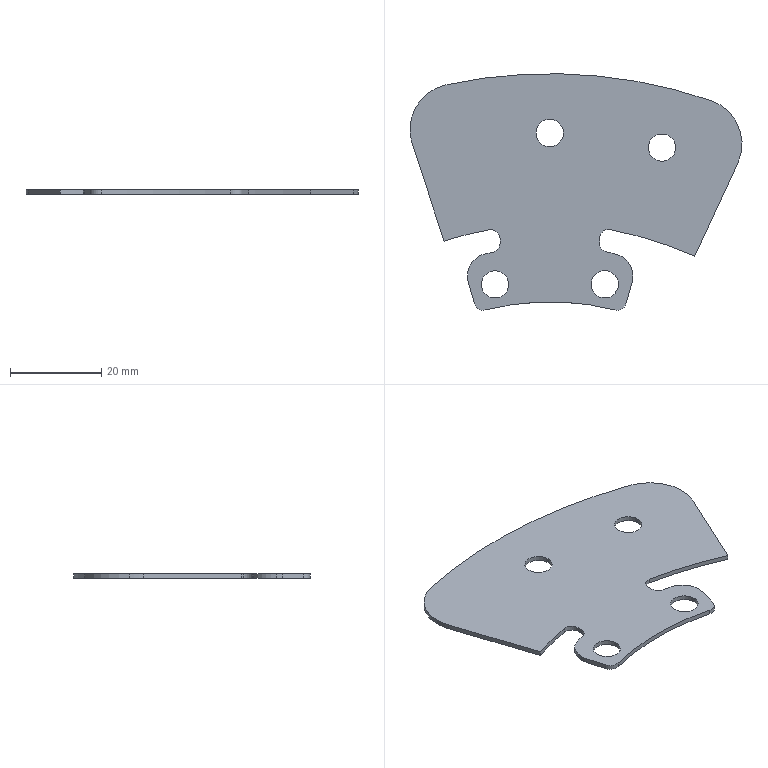Part | SolidWorks | features Extrusion 1 | 1 solid | 35 faces | box 72.756 x 51.823 x 1 mm | volume 2634 mm3 | cylinder 27 | plane 8 | commonest cylinder face diameters 6 x8 4 x7 10 x3 20 x3 140 x2 116 x1
STEP:
#1=CARTESIAN_POINT('',(21.592,11.76,1.));
#2=VERTEX_POINT('',#1);
#3=CARTESIAN_POINT('',(27.592,11.76,1.));
#4=VERTEX_POINT('',#3);
#5=CARTESIAN_POINT('',(24.592,11.76,1.));
#6=DIRECTION('',(0.,0.,1.));
#7=DIRECTION('',(1.,0.,0.));
#8=AXIS2_PLACEMENT_3D('',#5,#6,#7);
#9=CIRCLE('',#8,3.);
#10=EDGE_CURVE('',#2,#4,#9,.T.);
#11=ORIENTED_EDGE('',*,*,#10,.T.);
#12=CARTESIAN_POINT('',(27.592,11.76,0.));
#13=VERTEX_POINT('',#12);
#14=CARTESIAN_POINT('',(27.592,11.76,1.));
#15=DIRECTION('',(0.,0.,-1.));
#16=VECTOR('',#15,1000.);
#17=LINE('',#14,#16);
#18=EDGE_CURVE('',#4,#13,#17,.T.);
#19=ORIENTED_EDGE('',*,*,#18,.T.);
#20=CARTESIAN_POINT('',(21.592,11.76,0.));
#21=VERTEX_POINT('',#20);
#22=CARTESIAN_POINT('',(24.592,11.76,0.));
#23=DIRECTION('',(0.,0.,1.));
#24=DIRECTION('',(1.,0.,0.));
#25=AXIS2_PLACEMENT_3D('',#22,#23,#24);
#26=CIRCLE('',#25,3.);
#27=EDGE_CURVE('',#21,#13,#26,.T.);
#28=ORIENTED_EDGE('',*,*,#27,.F.);
#29=CARTESIAN_POINT('',(21.592,11.76,1.));
#30=DIRECTION('',(0.,0.,-1.));
#31=VECTOR('',#30,1000.);
#32=LINE('',#29,#31);
#33=EDGE_CURVE('',#2,#21,#32,.T.);
#34=ORIENTED_EDGE('',*,*,#33,.F.);
#35=EDGE_LOOP('',(#11,#19,#28,#34));
#36=FACE_OUTER_BOUND('',#35,.T.);
#37=CARTESIAN_POINT('',(24.592,11.76,1.));
#38=DIRECTION('',(0.,0.,-1.));
#39=DIRECTION('',(-1.,0.,0.));
#40=AXIS2_PLACEMENT_3D('',#37,#38,#39);
#41=CYLINDRICAL_SURFACE('',#40,3.);
#42=ADVANCED_FACE('',(#36),#41,.F.);
#43=CARTESIAN_POINT('',(-3.,14.968,1.));
#44=VERTEX_POINT('',#43);
#45=CARTESIAN_POINT('',(3.,14.968,1.));
#46=VERTEX_POINT('',#45);
#47=CARTESIAN_POINT('',(0.,14.968,1.));
#48=DIRECTION('',(0.,0.,1.));
#49=DIRECTION('',(1.,0.,0.));
#50=AXIS2_PLACEMENT_3D('',#47,#48,#49);
#51=CIRCLE('',#50,3.);
#52=EDGE_CURVE('',#44,#46,#51,.T.);
#53=ORIENTED_EDGE('',*,*,#52,.T.);
#54=CARTESIAN_POINT('',(3.,14.968,0.));
#55=VERTEX_POINT('',#54);
#56=CARTESIAN_POINT('',(3.,14.968,1.));
#57=DIRECTION('',(0.,0.,-1.));
#58=VECTOR('',#57,1000.);
#59=LINE('',#56,#58);
#60=EDGE_CURVE('',#46,#55,#59,.T.);
#61=ORIENTED_EDGE('',*,*,#60,.T.);
#62=CARTESIAN_POINT('',(-3.,14.968,0.));
#63=VERTEX_POINT('',#62);
#64=CARTESIAN_POINT('',(0.,14.968,0.));
#65=DIRECTION('',(0.,0.,1.));
#66=DIRECTION('',(1.,0.,0.));
#67=AXIS2_PLACEMENT_3D('',#64,#65,#66);
#68=CIRCLE('',#67,3.);
#69=EDGE_CURVE('',#63,#55,#68,.T.);
#70=ORIENTED_EDGE('',*,*,#69,.F.);
#71=CARTESIAN_POINT('',(-3.,14.968,1.));
#72=DIRECTION('',(0.,0.,-1.));
#73=VECTOR('',#72,1000.);
#74=LINE('',#71,#73);
#75=EDGE_CURVE('',#44,#63,#74,.T.);
#76=ORIENTED_EDGE('',*,*,#75,.F.);
#77=EDGE_LOOP('',(#53,#61,#70,#76));
#78=FACE_OUTER_BOUND('',#77,.T.);
#79=CARTESIAN_POINT('',(0.,14.968,1.));
#80=DIRECTION('',(0.,0.,-1.));
#81=DIRECTION('',(-1.,0.,0.));
#82=AXIS2_PLACEMENT_3D('',#79,#80,#81);
#83=CYLINDRICAL_SURFACE('',#82,3.);
#84=ADVANCED_FACE('',(#78),#83,.F.);
#85=CARTESIAN_POINT('',(-14.981,-18.204,1.));
#86=VERTEX_POINT('',#85);
#87=CARTESIAN_POINT('',(-8.981,-18.204,1.));
#88=VERTEX_POINT('',#87);
#89=CARTESIAN_POINT('',(-11.981,-18.204,1.));
#90=DIRECTION('',(0.,0.,1.));
#91=DIRECTION('',(1.,0.,0.));
#92=AXIS2_PLACEMENT_3D('',#89,#90,#91);
#93=CIRCLE('',#92,3.);
#94=EDGE_CURVE('',#86,#88,#93,.T.);
#95=ORIENTED_EDGE('',*,*,#94,.T.);
#96=CARTESIAN_POINT('',(-8.981,-18.204,0.));
#97=VERTEX_POINT('',#96);
#98=CARTESIAN_POINT('',(-8.981,-18.204,1.));
#99=DIRECTION('',(0.,0.,-1.));
#100=VECTOR('',#99,1000.);
#101=LINE('',#98,#100);
#102=EDGE_CURVE('',#88,#97,#101,.T.);
#103=ORIENTED_EDGE('',*,*,#102,.T.);
#104=CARTESIAN_POINT('',(-14.981,-18.204,0.));
#105=VERTEX_POINT('',#104);
#106=CARTESIAN_POINT('',(-11.981,-18.204,0.));
#107=DIRECTION('',(0.,0.,1.));
#108=DIRECTION('',(1.,0.,0.));
#109=AXIS2_PLACEMENT_3D('',#106,#107,#108);
#110=CIRCLE('',#109,3.);
#111=EDGE_CURVE('',#105,#97,#110,.T.);
#112=ORIENTED_EDGE('',*,*,#111,.F.);
#113=CARTESIAN_POINT('',(-14.981,-18.204,1.));
#114=DIRECTION('',(0.,0.,-1.));
#115=VECTOR('',#114,1000.);
#116=LINE('',#113,#115);
#117=EDGE_CURVE('',#86,#105,#116,.T.);
#118=ORIENTED_EDGE('',*,*,#117,.F.);
#119=EDGE_LOOP('',(#95,#103,#112,#118));
#120=FACE_OUTER_BOUND('',#119,.T.);
#121=CARTESIAN_POINT('',(-11.981,-18.204,1.));
#122=DIRECTION('',(0.,0.,-1.));
#123=DIRECTION('',(-1.,0.,0.));
#124=AXIS2_PLACEMENT_3D('',#121,#122,#123);
#125=CYLINDRICAL_SURFACE('',#124,3.);
#126=ADVANCED_FACE('',(#120),#125,.F.);
#127=CARTESIAN_POINT('',(9.061,-18.175,1.));
#128=VERTEX_POINT('',#127);
#129=CARTESIAN_POINT('',(15.061,-18.175,1.));
#130=VERTEX_POINT('',#129);
#131=CARTESIAN_POINT('',(12.061,-18.175,1.));
#132=DIRECTION('',(0.,0.,1.));
#133=DIRECTION('',(1.,0.,0.));
#134=AXIS2_PLACEMENT_3D('',#131,#132,#133);
#135=CIRCLE('',#134,3.);
#136=EDGE_CURVE('',#128,#130,#135,.T.);
#137=ORIENTED_EDGE('',*,*,#136,.T.);
#138=CARTESIAN_POINT('',(15.061,-18.175,0.));
#139=VERTEX_POINT('',#138);
#140=CARTESIAN_POINT('',(15.061,-18.175,1.));
#141=DIRECTION('',(0.,0.,-1.));
#142=VECTOR('',#141,1000.);
#143=LINE('',#140,#142);
#144=EDGE_CURVE('',#130,#139,#143,.T.);
#145=ORIENTED_EDGE('',*,*,#144,.T.);
#146=CARTESIAN_POINT('',(9.061,-18.175,0.));
#147=VERTEX_POINT('',#146);
#148=CARTESIAN_POINT('',(12.061,-18.175,0.));
#149=DIRECTION('',(0.,0.,1.));
#150=DIRECTION('',(1.,0.,0.));
#151=AXIS2_PLACEMENT_3D('',#148,#149,#150);
#152=CIRCLE('',#151,3.);
#153=EDGE_CURVE('',#147,#139,#152,.T.);
#154=ORIENTED_EDGE('',*,*,#153,.F.);
#155=CARTESIAN_POINT('',(9.061,-18.175,1.));
#156=DIRECTION('',(0.,0.,-1.));
#157=VECTOR('',#156,1000.);
#158=LINE('',#155,#157);
#159=EDGE_CURVE('',#128,#147,#158,.T.);
#160=ORIENTED_EDGE('',*,*,#159,.F.);
#161=EDGE_LOOP('',(#137,#145,#154,#160));
#162=FACE_OUTER_BOUND('',#161,.T.);
#163=CARTESIAN_POINT('',(12.061,-18.175,1.));
#164=DIRECTION('',(0.,0.,-1.));
#165=DIRECTION('',(-1.,0.,0.));
#166=AXIS2_PLACEMENT_3D('',#163,#164,#165);
#167=CYLINDRICAL_SURFACE('',#166,3.);
#168=ADVANCED_FACE('',(#162),#167,.F.);
#169=CARTESIAN_POINT('',(10.942,-8.168,1.));
#170=VERTEX_POINT('',#169);
#171=CARTESIAN_POINT('',(13.293,-6.199,1.));
#172=VERTEX_POINT('',#171);
#173=CARTESIAN_POINT('',(12.942,-8.168,1.));
#174=DIRECTION('',(0.,0.,-1.));
#175=DIRECTION('',(1.,0.,0.));
#176=AXIS2_PLACEMENT_3D('',#173,#174,#175);
#177=CIRCLE('',#176,2.);
#178=EDGE_CURVE('',#170,#172,#177,.T.);
#179=ORIENTED_EDGE('',*,*,#178,.F.);
#180=CARTESIAN_POINT('',(10.942,-8.168,0.));
#181=VERTEX_POINT('',#180);
#182=CARTESIAN_POINT('',(10.942,-8.168,1.));
#183=DIRECTION('',(0.,0.,-1.));
#184=VECTOR('',#183,1000.);
#185=LINE('',#182,#184);
#186=EDGE_CURVE('',#170,#181,#185,.T.);
#187=ORIENTED_EDGE('',*,*,#186,.T.);
#188=CARTESIAN_POINT('',(13.293,-6.199,0.));
#189=VERTEX_POINT('',#188);
#190=CARTESIAN_POINT('',(12.942,-8.168,0.));
#191=DIRECTION('',(0.,0.,-1.));
#192=DIRECTION('',(1.,0.,0.));
#193=AXIS2_PLACEMENT_3D('',#190,#191,#192);
#194=CIRCLE('',#193,2.);
#195=EDGE_CURVE('',#181,#189,#194,.T.);
#196=ORIENTED_EDGE('',*,*,#195,.T.);
#197=CARTESIAN_POINT('',(13.293,-6.199,1.));
#198=DIRECTION('',(0.,0.,-1.));
#199=VECTOR('',#198,1000.);
#200=LINE('',#197,#199);
#201=EDGE_CURVE('',#172,#189,#200,.T.);
#202=ORIENTED_EDGE('',*,*,#201,.F.);
#203=EDGE_LOOP('',(#179,#187,#196,#202));
#204=FACE_OUTER_BOUND('',#203,.T.);
#205=CARTESIAN_POINT('',(12.942,-8.168,1.));
#206=DIRECTION('',(0.,0.,-1.));
#207=DIRECTION('',(-1.,0.,0.));
#208=AXIS2_PLACEMENT_3D('',#205,#206,#207);
#209=CYLINDRICAL_SURFACE('',#208,2.);
#210=ADVANCED_FACE('',(#204),#209,.F.);
#211=CARTESIAN_POINT('',(-18.02,-16.372,1.));
#212=VERTEX_POINT('',#211);
#213=CARTESIAN_POINT('',(-17.824,-17.756,1.));
#214=VERTEX_POINT('',#213);
#215=CARTESIAN_POINT('',(-13.02,-16.372,1.));
#216=DIRECTION('',(0.,0.,1.));
#217=DIRECTION('',(1.,0.,0.));
#218=AXIS2_PLACEMENT_3D('',#215,#216,#217);
#219=CIRCLE('',#218,5.);
#220=EDGE_CURVE('',#212,#214,#219,.T.);
#221=ORIENTED_EDGE('',*,*,#220,.F.);
#222=CARTESIAN_POINT('',(-18.02,-16.372,0.));
#223=VERTEX_POINT('',#222);
#224=CARTESIAN_POINT('',(-18.02,-16.372,1.));
#225=DIRECTION('',(0.,0.,-1.));
#226=VECTOR('',#225,1000.);
#227=LINE('',#224,#226);
#228=EDGE_CURVE('',#212,#223,#227,.T.);
#229=ORIENTED_EDGE('',*,*,#228,.T.);
#230=CARTESIAN_POINT('',(-17.824,-17.756,0.));
#231=VERTEX_POINT('',#230);
#232=CARTESIAN_POINT('',(-13.02,-16.372,0.));
#233=DIRECTION('',(0.,0.,1.));
#234=DIRECTION('',(1.,0.,0.));
#235=AXIS2_PLACEMENT_3D('',#232,#233,#234);
#236=CIRCLE('',#235,5.);
#237=EDGE_CURVE('',#223,#231,#236,.T.);
#238=ORIENTED_EDGE('',*,*,#237,.T.);
#239=CARTESIAN_POINT('',(-17.824,-17.756,1.));
#240=DIRECTION('',(0.,0.,-1.));
#241=VECTOR('',#240,1000.);
#242=LINE('',#239,#241);
#243=EDGE_CURVE('',#214,#231,#242,.T.);
#244=ORIENTED_EDGE('',*,*,#243,.F.);
#245=EDGE_LOOP('',(#221,#229,#238,#244));
#246=FACE_OUTER_BOUND('',#245,.T.);
#247=CARTESIAN_POINT('',(-13.02,-16.372,1.));
#248=DIRECTION('',(0.,0.,-1.));
#249=DIRECTION('',(-1.,0.,0.));
#250=AXIS2_PLACEMENT_3D('',#247,#248,#249);
#251=CYLINDRICAL_SURFACE('',#250,5.);
#252=ADVANCED_FACE('',(#246),#251,.T.);
#253=CARTESIAN_POINT('',(-30.616,15.751,1.));
#254=VERTEX_POINT('',#253);
#255=CARTESIAN_POINT('',(-30.123,12.649,1.));
#256=VERTEX_POINT('',#255);
#257=CARTESIAN_POINT('',(-20.616,15.751,1.));
#258=DIRECTION('',(0.,0.,1.));
#259=DIRECTION('',(1.,0.,0.));
#260=AXIS2_PLACEMENT_3D('',#257,#258,#259);
#261=CIRCLE('',#260,10.);
#262=EDGE_CURVE('',#254,#256,#261,.T.);
#263=ORIENTED_EDGE('',*,*,#262,.F.);
#264=CARTESIAN_POINT('',(-30.616,15.751,0.));
#265=VERTEX_POINT('',#264);
#266=CARTESIAN_POINT('',(-30.616,15.751,1.));
#267=DIRECTION('',(0.,0.,-1.));
#268=VECTOR('',#267,1000.);
#269=LINE('',#266,#268);
#270=EDGE_CURVE('',#254,#265,#269,.T.);
#271=ORIENTED_EDGE('',*,*,#270,.T.);
#272=CARTESIAN_POINT('',(-30.123,12.649,0.));
#273=VERTEX_POINT('',#272);
#274=CARTESIAN_POINT('',(-20.616,15.751,0.));
#275=DIRECTION('',(0.,0.,1.));
#276=DIRECTION('',(1.,0.,0.));
#277=AXIS2_PLACEMENT_3D('',#274,#275,#276);
#278=CIRCLE('',#277,10.);
#279=EDGE_CURVE('',#265,#273,#278,.T.);
#280=ORIENTED_EDGE('',*,*,#279,.T.);
#281=CARTESIAN_POINT('',(-30.123,12.649,1.));
#282=DIRECTION('',(0.,0.,-1.));
#283=VECTOR('',#282,1000.);
#284=LINE('',#281,#283);
#285=EDGE_CURVE('',#256,#273,#284,.T.);
#286=ORIENTED_EDGE('',*,*,#285,.F.);
#287=EDGE_LOOP('',(#263,#271,#280,#286));
#288=FACE_OUTER_BOUND('',#287,.T.);
#289=CARTESIAN_POINT('',(-20.616,15.751,1.));
#290=DIRECTION('',(0.,0.,-1.));
#291=DIRECTION('',(-1.,0.,0.));
#292=AXIS2_PLACEMENT_3D('',#289,#290,#291);
#293=CYLINDRICAL_SURFACE('',#292,10.);
#294=ADVANCED_FACE('',(#288),#293,.T.);
#295=ORIENTED_EDGE('',*,*,#52,.F.);
#296=CARTESIAN_POINT('',(0.,14.968,1.));
#297=DIRECTION('',(0.,0.,1.));
#298=DIRECTION('',(1.,0.,0.));
#299=AXIS2_PLACEMENT_3D('',#296,#297,#298);
#300=CIRCLE('',#299,3.);
#301=EDGE_CURVE('',#46,#44,#300,.T.);
#302=ORIENTED_EDGE('',*,*,#301,.F.);
#303=EDGE_LOOP('',(#295,#302));
#304=FACE_BOUND('',#303,.T.);
#305=ORIENTED_EDGE('',*,*,#136,.F.);
#306=CARTESIAN_POINT('',(12.061,-18.175,1.));
#307=DIRECTION('',(0.,0.,1.));
#308=DIRECTION('',(1.,0.,0.));
#309=AXIS2_PLACEMENT_3D('',#306,#307,#308);
#310=CIRCLE('',#309,3.);
#311=EDGE_CURVE('',#130,#128,#310,.T.);
#312=ORIENTED_EDGE('',*,*,#311,.F.);
#313=EDGE_LOOP('',(#305,#312));
#314=FACE_BOUND('',#313,.T.);
#315=CARTESIAN_POINT('',(41.208,8.372,1.));
#316=VERTEX_POINT('',#315);
#317=CARTESIAN_POINT('',(35.408,22.038,1.));
#318=VERTEX_POINT('',#317);
#319=CARTESIAN_POINT('',(32.14,12.587,1.));
#320=DIRECTION('',(0.,0.,1.));
#321=DIRECTION('',(1.,0.,0.));
#322=AXIS2_PLACEMENT_3D('',#319,#320,#321);
#323=CIRCLE('',#322,10.);
#324=EDGE_CURVE('',#316,#318,#323,.T.);
#325=ORIENTED_EDGE('',*,*,#324,.T.);
#326=CARTESIAN_POINT('',(-22.731,25.524,1.));
#327=VERTEX_POINT('',#326);
#328=CARTESIAN_POINT('',(0.1133,-80.032,1.));
#329=DIRECTION('',(0.,0.,1.));
#330=DIRECTION('',(1.,0.,0.));
#331=AXIS2_PLACEMENT_3D('',#328,#329,#330);
#332=CIRCLE('',#331,108.);
#333=EDGE_CURVE('',#318,#327,#332,.T.);
#334=ORIENTED_EDGE('',*,*,#333,.T.);
#335=CARTESIAN_POINT('',(-20.616,15.751,1.));
#336=DIRECTION('',(0.,0.,1.));
#337=DIRECTION('',(1.,0.,0.));
#338=AXIS2_PLACEMENT_3D('',#335,#336,#337);
#339=CIRCLE('',#338,10.);
#340=EDGE_CURVE('',#327,#254,#339,.T.);
#341=ORIENTED_EDGE('',*,*,#340,.T.);
#342=ORIENTED_EDGE('',*,*,#262,.T.);
#343=CARTESIAN_POINT('',(-23.148,-8.73,1.));
#344=VERTEX_POINT('',#343);
#345=CARTESIAN_POINT('',(-23.148,-8.73,1.));
#346=DIRECTION('',(0.3102,-0.9507,0.));
#347=VECTOR('',#346,1000.);
#348=LINE('',#345,#347);
#349=EDGE_CURVE('',#256,#344,#348,.T.);
#350=ORIENTED_EDGE('',*,*,#349,.T.);
#351=CARTESIAN_POINT('',(-13.243,-6.231,1.));
#352=VERTEX_POINT('',#351);
#353=CARTESIAN_POINT('',(0.1133,-80.032,1.));
#354=DIRECTION('',(0.,0.,-1.));
#355=DIRECTION('',(1.,0.,0.));
#356=AXIS2_PLACEMENT_3D('',#353,#354,#355);
#357=CIRCLE('',#356,75.);
#358=EDGE_CURVE('',#344,#352,#357,.T.);
#359=ORIENTED_EDGE('',*,*,#358,.T.);
#360=CARTESIAN_POINT('',(-10.887,-8.199,1.));
#361=VERTEX_POINT('',#360);
#362=CARTESIAN_POINT('',(-12.887,-8.199,1.));
#363=DIRECTION('',(0.,0.,-1.));
#364=DIRECTION('',(1.,0.,0.));
#365=AXIS2_PLACEMENT_3D('',#362,#363,#364);
#366=CIRCLE('',#365,2.);
#367=EDGE_CURVE('',#352,#361,#366,.T.);
#368=ORIENTED_EDGE('',*,*,#367,.T.);
#369=CARTESIAN_POINT('',(-10.887,-9.215,1.));
#370=VERTEX_POINT('',#369);
#371=CARTESIAN_POINT('',(-10.887,-8.199,1.));
#372=DIRECTION('',(0.,-1.,0.));
#373=VECTOR('',#372,1000.);
#374=LINE('',#371,#373);
#375=EDGE_CURVE('',#361,#370,#374,.T.);
#376=ORIENTED_EDGE('',*,*,#375,.T.);
#377=CARTESIAN_POINT('',(-12.526,-11.182,1.));
#378=VERTEX_POINT('',#377);
#379=CARTESIAN_POINT('',(-12.887,-9.215,1.));
#380=DIRECTION('',(0.,0.,-1.));
#381=DIRECTION('',(1.,0.,0.));
#382=AXIS2_PLACEMENT_3D('',#379,#380,#381);
#383=CIRCLE('',#382,2.);
#384=EDGE_CURVE('',#370,#378,#383,.T.);
#385=ORIENTED_EDGE('',*,*,#384,.T.);
#386=CARTESIAN_POINT('',(-14.03,-11.475,1.));
#387=VERTEX_POINT('',#386);
#388=CARTESIAN_POINT('',(0.1133,-80.032,1.));
#389=DIRECTION('',(0.,0.,1.));
#390=DIRECTION('',(1.,0.,0.));
#391=AXIS2_PLACEMENT_3D('',#388,#389,#390);
#392=CIRCLE('',#391,70.);
#393=EDGE_CURVE('',#378,#387,#392,.T.);
#394=ORIENTED_EDGE('',*,*,#393,.T.);
#395=CARTESIAN_POINT('',(-13.02,-16.372,1.));
#396=DIRECTION('',(0.,0.,1.));
#397=DIRECTION('',(1.,0.,0.));
#398=AXIS2_PLACEMENT_3D('',#395,#396,#397);
#399=CIRCLE('',#398,5.);
#400=EDGE_CURVE('',#387,#212,#399,.T.);
#401=ORIENTED_EDGE('',*,*,#400,.T.);
#402=ORIENTED_EDGE('',*,*,#220,.T.);
#403=CARTESIAN_POINT('',(-16.484,-22.408,1.));
#404=VERTEX_POINT('',#403);
#405=CARTESIAN_POINT('',(-16.484,-22.408,1.));
#406=DIRECTION('',(0.2768,-0.9609,0.));
#407=VECTOR('',#406,1000.);
#408=LINE('',#405,#407);
#409=EDGE_CURVE('',#214,#404,#408,.T.);
#410=ORIENTED_EDGE('',*,*,#409,.T.);
#411=CARTESIAN_POINT('',(-14.073,-23.794,1.));
#412=VERTEX_POINT('',#411);
#413=CARTESIAN_POINT('',(-14.563,-21.854,1.));
#414=DIRECTION('',(0.,0.,1.));
#415=DIRECTION('',(1.,0.,0.));
#416=AXIS2_PLACEMENT_3D('',#413,#414,#415);
#417=CIRCLE('',#416,2.);
#418=EDGE_CURVE('',#404,#412,#417,.T.);
#419=ORIENTED_EDGE('',*,*,#418,.T.);
#420=CARTESIAN_POINT('',(14.3,-23.794,1.));
#421=VERTEX_POINT('',#420);
#422=CARTESIAN_POINT('',(0.1133,-80.032,1.));
#423=DIRECTION('',(0.,0.,-1.));
#424=DIRECTION('',(1.,0.,0.));
#425=AXIS2_PLACEMENT_3D('',#422,#423,#424);
#426=CIRCLE('',#425,58.);
#427=EDGE_CURVE('',#412,#421,#426,.T.);
#428=ORIENTED_EDGE('',*,*,#427,.T.);
#429=CARTESIAN_POINT('',(16.711,-22.408,1.));
#430=VERTEX_POINT('',#429);
#431=CARTESIAN_POINT('',(14.789,-21.854,1.));
#432=DIRECTION('',(0.,0.,1.));
#433=DIRECTION('',(1.,0.,0.));
#434=AXIS2_PLACEMENT_3D('',#431,#432,#433);
#435=CIRCLE('',#434,2.);
#436=EDGE_CURVE('',#421,#430,#435,.T.);
#437=ORIENTED_EDGE('',*,*,#436,.T.);
#438=CARTESIAN_POINT('',(18.051,-17.756,1.));
#439=VERTEX_POINT('',#438);
#440=CARTESIAN_POINT('',(16.711,-22.408,1.));
#441=DIRECTION('',(0.2768,0.9609,0.));
#442=VECTOR('',#441,1000.);
#443=LINE('',#440,#442);
#444=EDGE_CURVE('',#430,#439,#443,.T.);
#445=ORIENTED_EDGE('',*,*,#444,.T.);
#446=CARTESIAN_POINT('',(14.257,-11.475,1.));
#447=VERTEX_POINT('',#446);
#448=CARTESIAN_POINT('',(13.246,-16.372,1.));
#449=DIRECTION('',(0.,0.,1.));
#450=DIRECTION('',(1.,0.,0.));
#451=AXIS2_PLACEMENT_3D('',#448,#449,#450);
#452=CIRCLE('',#451,5.);
#453=EDGE_CURVE('',#439,#447,#452,.T.);
#454=ORIENTED_EDGE('',*,*,#453,.T.);
#455=CARTESIAN_POINT('',(12.588,-11.152,1.));
#456=VERTEX_POINT('',#455);
#457=CARTESIAN_POINT('',(0.1133,-80.032,1.));
#458=DIRECTION('',(0.,0.,1.));
#459=DIRECTION('',(1.,0.,0.));
#460=AXIS2_PLACEMENT_3D('',#457,#458,#459);
#461=CIRCLE('',#460,70.);
#462=EDGE_CURVE('',#447,#456,#461,.T.);
#463=ORIENTED_EDGE('',*,*,#462,.T.);
#464=CARTESIAN_POINT('',(10.944,-9.189,1.));
#465=VERTEX_POINT('',#464);
#466=CARTESIAN_POINT('',(12.944,-9.184,1.));
#467=DIRECTION('',(0.,0.,-1.));
#468=DIRECTION('',(1.,0.,0.));
#469=AXIS2_PLACEMENT_3D('',#466,#467,#468);
#470=CIRCLE('',#469,2.);
#471=EDGE_CURVE('',#456,#465,#470,.T.);
#472=ORIENTED_EDGE('',*,*,#471,.T.);
#473=CARTESIAN_POINT('',(10.942,-8.173,1.));
#474=VERTEX_POINT('',#473);
#475=CARTESIAN_POINT('',(10.942,-8.173,1.));
#476=DIRECTION('',(-0.002386,1.,0.));
#477=VECTOR('',#476,1000.);
#478=LINE('',#475,#477);
#479=EDGE_CURVE('',#465,#474,#478,.T.);
#480=ORIENTED_EDGE('',*,*,#479,.T.);
#481=CARTESIAN_POINT('',(12.942,-8.168,1.));
#482=DIRECTION('',(0.,0.,-1.));
#483=DIRECTION('',(1.,0.,0.));
#484=AXIS2_PLACEMENT_3D('',#481,#482,#483);
#485=CIRCLE('',#484,2.);
#486=EDGE_CURVE('',#474,#170,#485,.T.);
#487=ORIENTED_EDGE('',*,*,#486,.T.);
#488=ORIENTED_EDGE('',*,*,#178,.T.);
#489=CARTESIAN_POINT('',(31.729,-12.021,1.));
#490=VERTEX_POINT('',#489);
#491=CARTESIAN_POINT('',(-3.673,-92.021,1.));
#492=DIRECTION('',(0.,0.,-1.));
#493=DIRECTION('',(1.,0.,0.));
#494=AXIS2_PLACEMENT_3D('',#491,#492,#493);
#495=CIRCLE('',#494,87.483);
#496=EDGE_CURVE('',#172,#490,#495,.T.);
#497=ORIENTED_EDGE('',*,*,#496,.T.);
#498=CARTESIAN_POINT('',(31.729,-12.021,1.));
#499=DIRECTION('',(0.4215,0.9068,0.));
#500=VECTOR('',#499,1000.);
#501=LINE('',#498,#500);
#502=EDGE_CURVE('',#490,#316,#501,.T.);
#503=ORIENTED_EDGE('',*,*,#502,.T.);
#504=EDGE_LOOP('',(#325,#334,#341,#342,#350,#359,#368,#376,#385,#394,#401,#402,#410,#419,#428,#437,#445,#454,#463,#472,#480,#487,#488,#497,#503));
#505=FACE_OUTER_BOUND('',#504,.T.);
#506=ORIENTED_EDGE('',*,*,#94,.F.);
#507=CARTESIAN_POINT('',(-11.981,-18.204,1.));
#508=DIRECTION('',(0.,0.,1.));
#509=DIRECTION('',(1.,0.,0.));
#510=AXIS2_PLACEMENT_3D('',#507,#508,#509);
#511=CIRCLE('',#510,3.);
#512=EDGE_CURVE('',#88,#86,#511,.T.);
#513=ORIENTED_EDGE('',*,*,#512,.F.);
#514=EDGE_LOOP('',(#506,#513));
#515=FACE_BOUND('',#514,.T.);
#516=ORIENTED_EDGE('',*,*,#10,.F.);
#517=CARTESIAN_POINT('',(24.592,11.76,1.));
#518=DIRECTION('',(0.,0.,1.));
#519=DIRECTION('',(1.,0.,0.));
#520=AXIS2_PLACEMENT_3D('',#517,#518,#519);
#521=CIRCLE('',#520,3.);
#522=EDGE_CURVE('',#4,#2,#521,.T.);
#523=ORIENTED_EDGE('',*,*,#522,.F.);
#524=EDGE_LOOP('',(#516,#523));
#525=FACE_BOUND('',#524,.T.);
#526=CARTESIAN_POINT('',(32.14,12.587,1.));
#527=DIRECTION('',(0.,0.,1.));
#528=DIRECTION('',(1.,0.,0.));
#529=AXIS2_PLACEMENT_3D('',#526,#527,#528);
#530=PLANE('',#529);
#531=ADVANCED_FACE('',(#304,#314,#505,#515,#525),#530,.T.);
#532=CARTESIAN_POINT('',(41.208,8.372,0.));
#533=VERTEX_POINT('',#532);
#534=CARTESIAN_POINT('',(35.408,22.038,0.));
#535=VERTEX_POINT('',#534);
#536=CARTESIAN_POINT('',(32.14,12.587,0.));
#537=DIRECTION('',(0.,0.,1.));
#538=DIRECTION('',(1.,0.,0.));
#539=AXIS2_PLACEMENT_3D('',#536,#537,#538);
#540=CIRCLE('',#539,10.);
#541=EDGE_CURVE('',#533,#535,#540,.T.);
#542=ORIENTED_EDGE('',*,*,#541,.F.);
#543=CARTESIAN_POINT('',(31.729,-12.021,0.));
#544=VERTEX_POINT('',#543);
#545=CARTESIAN_POINT('',(31.729,-12.021,0.));
#546=DIRECTION('',(0.4215,0.9068,0.));
#547=VECTOR('',#546,1000.);
#548=LINE('',#545,#547);
#549=EDGE_CURVE('',#544,#533,#548,.T.);
#550=ORIENTED_EDGE('',*,*,#549,.F.);
#551=CARTESIAN_POINT('',(-3.673,-92.021,0.));
#552=DIRECTION('',(0.,0.,-1.));
#553=DIRECTION('',(1.,0.,0.));
#554=AXIS2_PLACEMENT_3D('',#551,#552,#553);
#555=CIRCLE('',#554,87.483);
#556=EDGE_CURVE('',#189,#544,#555,.T.);
#557=ORIENTED_EDGE('',*,*,#556,.F.);
#558=ORIENTED_EDGE('',*,*,#195,.F.);
#559=CARTESIAN_POINT('',(10.942,-8.173,0.));
#560=VERTEX_POINT('',#559);
#561=CARTESIAN_POINT('',(12.942,-8.168,0.));
#562=DIRECTION('',(0.,0.,-1.));
#563=DIRECTION('',(1.,0.,0.));
#564=AXIS2_PLACEMENT_3D('',#561,#562,#563);
#565=CIRCLE('',#564,2.);
#566=EDGE_CURVE('',#560,#181,#565,.T.);
#567=ORIENTED_EDGE('',*,*,#566,.F.);
#568=CARTESIAN_POINT('',(10.944,-9.189,0.));
#569=VERTEX_POINT('',#568);
#570=CARTESIAN_POINT('',(10.942,-8.173,0.));
#571=DIRECTION('',(-0.002386,1.,0.));
#572=VECTOR('',#571,1000.);
#573=LINE('',#570,#572);
#574=EDGE_CURVE('',#569,#560,#573,.T.);
#575=ORIENTED_EDGE('',*,*,#574,.F.);
#576=CARTESIAN_POINT('',(12.588,-11.152,0.));
#577=VERTEX_POINT('',#576);
#578=CARTESIAN_POINT('',(12.944,-9.184,0.));
#579=DIRECTION('',(0.,0.,-1.));
#580=DIRECTION('',(1.,0.,0.));
#581=AXIS2_PLACEMENT_3D('',#578,#579,#580);
#582=CIRCLE('',#581,2.);
#583=EDGE_CURVE('',#577,#569,#582,.T.);
#584=ORIENTED_EDGE('',*,*,#583,.F.);
#585=CARTESIAN_POINT('',(14.257,-11.475,0.));
#586=VERTEX_POINT('',#585);
#587=CARTESIAN_POINT('',(0.1133,-80.032,0.));
#588=DIRECTION('',(0.,0.,1.));
#589=DIRECTION('',(1.,0.,0.));
#590=AXIS2_PLACEMENT_3D('',#587,#588,#589);
#591=CIRCLE('',#590,70.);
#592=EDGE_CURVE('',#586,#577,#591,.T.);
#593=ORIENTED_EDGE('',*,*,#592,.F.);
#594=CARTESIAN_POINT('',(18.051,-17.756,0.));
#595=VERTEX_POINT('',#594);
#596=CARTESIAN_POINT('',(13.246,-16.372,0.));
#597=DIRECTION('',(0.,0.,1.));
#598=DIRECTION('',(1.,0.,0.));
#599=AXIS2_PLACEMENT_3D('',#596,#597,#598);
#600=CIRCLE('',#599,5.);
#601=EDGE_CURVE('',#595,#586,#600,.T.);
#602=ORIENTED_EDGE('',*,*,#601,.F.);
#603=CARTESIAN_POINT('',(16.711,-22.408,0.));
#604=VERTEX_POINT('',#603);
#605=CARTESIAN_POINT('',(16.711,-22.408,0.));
#606=DIRECTION('',(0.2768,0.9609,0.));
#607=VECTOR('',#606,1000.);
#608=LINE('',#605,#607);
#609=EDGE_CURVE('',#604,#595,#608,.T.);
#610=ORIENTED_EDGE('',*,*,#609,.F.);
#611=CARTESIAN_POINT('',(14.3,-23.794,0.));
#612=VERTEX_POINT('',#611);
#613=CARTESIAN_POINT('',(14.789,-21.854,0.));
#614=DIRECTION('',(0.,0.,1.));
#615=DIRECTION('',(1.,0.,0.));
#616=AXIS2_PLACEMENT_3D('',#613,#614,#615);
#617=CIRCLE('',#616,2.);
#618=EDGE_CURVE('',#612,#604,#617,.T.);
#619=ORIENTED_EDGE('',*,*,#618,.F.);
#620=CARTESIAN_POINT('',(-14.073,-23.794,0.));
#621=VERTEX_POINT('',#620);
#622=CARTESIAN_POINT('',(0.1133,-80.032,0.));
#623=DIRECTION('',(0.,0.,-1.));
#624=DIRECTION('',(1.,0.,0.));
#625=AXIS2_PLACEMENT_3D('',#622,#623,#624);
#626=CIRCLE('',#625,58.);
#627=EDGE_CURVE('',#621,#612,#626,.T.);
#628=ORIENTED_EDGE('',*,*,#627,.F.);
#629=CARTESIAN_POINT('',(-16.484,-22.408,0.));
#630=VERTEX_POINT('',#629);
#631=CARTESIAN_POINT('',(-14.563,-21.854,0.));
#632=DIRECTION('',(0.,0.,1.));
#633=DIRECTION('',(1.,0.,0.));
#634=AXIS2_PLACEMENT_3D('',#631,#632,#633);
#635=CIRCLE('',#634,2.);
#636=EDGE_CURVE('',#630,#621,#635,.T.);
#637=ORIENTED_EDGE('',*,*,#636,.F.);
#638=CARTESIAN_POINT('',(-16.484,-22.408,0.));
#639=DIRECTION('',(0.2768,-0.9609,0.));
#640=VECTOR('',#639,1000.);
#641=LINE('',#638,#640);
#642=EDGE_CURVE('',#231,#630,#641,.T.);
#643=ORIENTED_EDGE('',*,*,#642,.F.);
#644=ORIENTED_EDGE('',*,*,#237,.F.);
#645=CARTESIAN_POINT('',(-14.03,-11.475,0.));
#646=VERTEX_POINT('',#645);
#647=CARTESIAN_POINT('',(-13.02,-16.372,0.));
#648=DIRECTION('',(0.,0.,1.));
#649=DIRECTION('',(1.,0.,0.));
#650=AXIS2_PLACEMENT_3D('',#647,#648,#649);
#651=CIRCLE('',#650,5.);
#652=EDGE_CURVE('',#646,#223,#651,.T.);
#653=ORIENTED_EDGE('',*,*,#652,.F.);
#654=CARTESIAN_POINT('',(-12.526,-11.182,0.));
#655=VERTEX_POINT('',#654);
#656=CARTESIAN_POINT('',(0.1133,-80.032,0.));
#657=DIRECTION('',(0.,0.,1.));
#658=DIRECTION('',(1.,0.,0.));
#659=AXIS2_PLACEMENT_3D('',#656,#657,#658);
#660=CIRCLE('',#659,70.);
#661=EDGE_CURVE('',#655,#646,#660,.T.);
#662=ORIENTED_EDGE('',*,*,#661,.F.);
#663=CARTESIAN_POINT('',(-10.887,-9.215,0.));
#664=VERTEX_POINT('',#663);
#665=CARTESIAN_POINT('',(-12.887,-9.215,0.));
#666=DIRECTION('',(0.,0.,-1.));
#667=DIRECTION('',(1.,0.,0.));
#668=AXIS2_PLACEMENT_3D('',#665,#666,#667);
#669=CIRCLE('',#668,2.);
#670=EDGE_CURVE('',#664,#655,#669,.T.);
#671=ORIENTED_EDGE('',*,*,#670,.F.);
#672=CARTESIAN_POINT('',(-10.887,-8.199,0.));
#673=VERTEX_POINT('',#672);
#674=CARTESIAN_POINT('',(-10.887,-8.199,0.));
#675=DIRECTION('',(0.,-1.,0.));
#676=VECTOR('',#675,1000.);
#677=LINE('',#674,#676);
#678=EDGE_CURVE('',#673,#664,#677,.T.);
#679=ORIENTED_EDGE('',*,*,#678,.F.);
#680=CARTESIAN_POINT('',(-13.243,-6.231,0.));
#681=VERTEX_POINT('',#680);
#682=CARTESIAN_POINT('',(-12.887,-8.199,0.));
#683=DIRECTION('',(0.,0.,-1.));
#684=DIRECTION('',(1.,0.,0.));
#685=AXIS2_PLACEMENT_3D('',#682,#683,#684);
#686=CIRCLE('',#685,2.);
#687=EDGE_CURVE('',#681,#673,#686,.T.);
#688=ORIENTED_EDGE('',*,*,#687,.F.);
#689=CARTESIAN_POINT('',(-23.148,-8.73,0.));
#690=VERTEX_POINT('',#689);
#691=CARTESIAN_POINT('',(0.1133,-80.032,0.));
#692=DIRECTION('',(0.,0.,-1.));
#693=DIRECTION('',(1.,0.,0.));
#694=AXIS2_PLACEMENT_3D('',#691,#692,#693);
#695=CIRCLE('',#694,75.);
#696=EDGE_CURVE('',#690,#681,#695,.T.);
#697=ORIENTED_EDGE('',*,*,#696,.F.);
#698=CARTESIAN_POINT('',(-23.148,-8.73,0.));
#699=DIRECTION('',(0.3102,-0.9507,0.));
#700=VECTOR('',#699,1000.);
#701=LINE('',#698,#700);
#702=EDGE_CURVE('',#273,#690,#701,.T.);
#703=ORIENTED_EDGE('',*,*,#702,.F.);
#704=ORIENTED_EDGE('',*,*,#279,.F.);
#705=CARTESIAN_POINT('',(-22.731,25.524,0.));
#706=VERTEX_POINT('',#705);
#707=CARTESIAN_POINT('',(-20.616,15.751,0.));
#708=DIRECTION('',(0.,0.,1.));
#709=DIRECTION('',(1.,0.,0.));
#710=AXIS2_PLACEMENT_3D('',#707,#708,#709);
#711=CIRCLE('',#710,10.);
#712=EDGE_CURVE('',#706,#265,#711,.T.);
#713=ORIENTED_EDGE('',*,*,#712,.F.);
#714=CARTESIAN_POINT('',(0.1133,-80.032,0.));
#715=DIRECTION('',(0.,0.,1.));
#716=DIRECTION('',(1.,0.,0.));
#717=AXIS2_PLACEMENT_3D('',#714,#715,#716);
#718=CIRCLE('',#717,108.);
#719=EDGE_CURVE('',#535,#706,#718,.T.);
#720=ORIENTED_EDGE('',*,*,#719,.F.);
#721=EDGE_LOOP('',(#542,#550,#557,#558,#567,#575,#584,#593,#602,#610,#619,#628,#637,#643,#644,#653,#662,#671,#679,#688,#697,#703,#704,#713,#720));
#722=FACE_OUTER_BOUND('',#721,.T.);
#723=ORIENTED_EDGE('',*,*,#153,.T.);
#724=CARTESIAN_POINT('',(12.061,-18.175,0.));
#725=DIRECTION('',(0.,0.,1.));
#726=DIRECTION('',(1.,0.,0.));
#727=AXIS2_PLACEMENT_3D('',#724,#725,#726);
#728=CIRCLE('',#727,3.);
#729=EDGE_CURVE('',#139,#147,#728,.T.);
#730=ORIENTED_EDGE('',*,*,#729,.T.);
#731=EDGE_LOOP('',(#723,#730));
#732=FACE_BOUND('',#731,.T.);
#733=ORIENTED_EDGE('',*,*,#111,.T.);
#734=CARTESIAN_POINT('',(-11.981,-18.204,0.));
#735=DIRECTION('',(0.,0.,1.));
#736=DIRECTION('',(1.,0.,0.));
#737=AXIS2_PLACEMENT_3D('',#734,#735,#736);
#738=CIRCLE('',#737,3.);
#739=EDGE_CURVE('',#97,#105,#738,.T.);
#740=ORIENTED_EDGE('',*,*,#739,.T.);
#741=EDGE_LOOP('',(#733,#740));
#742=FACE_BOUND('',#741,.T.);
#743=ORIENTED_EDGE('',*,*,#69,.T.);
#744=CARTESIAN_POINT('',(0.,14.968,0.));
#745=DIRECTION('',(0.,0.,1.));
#746=DIRECTION('',(1.,0.,0.));
#747=AXIS2_PLACEMENT_3D('',#744,#745,#746);
#748=CIRCLE('',#747,3.);
#749=EDGE_CURVE('',#55,#63,#748,.T.);
#750=ORIENTED_EDGE('',*,*,#749,.T.);
#751=EDGE_LOOP('',(#743,#750));
#752=FACE_BOUND('',#751,.T.);
#753=ORIENTED_EDGE('',*,*,#27,.T.);
#754=CARTESIAN_POINT('',(24.592,11.76,0.));
#755=DIRECTION('',(0.,0.,1.));
#756=DIRECTION('',(1.,0.,0.));
#757=AXIS2_PLACEMENT_3D('',#754,#755,#756);
#758=CIRCLE('',#757,3.);
#759=EDGE_CURVE('',#13,#21,#758,.T.);
#760=ORIENTED_EDGE('',*,*,#759,.T.);
#761=EDGE_LOOP('',(#753,#760));
#762=FACE_BOUND('',#761,.T.);
#763=CARTESIAN_POINT('',(32.14,12.587,0.));
#764=DIRECTION('',(0.,0.,1.));
#765=DIRECTION('',(1.,0.,0.));
#766=AXIS2_PLACEMENT_3D('',#763,#764,#765);
#767=PLANE('',#766);
#768=ADVANCED_FACE('',(#722,#732,#742,#752,#762),#767,.F.);
#769=ORIENTED_EDGE('',*,*,#541,.T.);
#770=CARTESIAN_POINT('',(35.408,22.038,1.));
#771=DIRECTION('',(0.,0.,-1.));
#772=VECTOR('',#771,1000.);
#773=LINE('',#770,#772);
#774=EDGE_CURVE('',#318,#535,#773,.T.);
#775=ORIENTED_EDGE('',*,*,#774,.F.);
#776=ORIENTED_EDGE('',*,*,#324,.F.);
#777=CARTESIAN_POINT('',(41.208,8.372,1.));
#778=DIRECTION('',(0.,0.,-1.));
#779=VECTOR('',#778,1000.);
#780=LINE('',#777,#779);
#781=EDGE_CURVE('',#316,#533,#780,.T.);
#782=ORIENTED_EDGE('',*,*,#781,.T.);
#783=EDGE_LOOP('',(#769,#775,#776,#782));
#784=FACE_OUTER_BOUND('',#783,.T.);
#785=CARTESIAN_POINT('',(32.14,12.587,1.));
#786=DIRECTION('',(0.,0.,-1.));
#787=DIRECTION('',(-1.,0.,0.));
#788=AXIS2_PLACEMENT_3D('',#785,#786,#787);
#789=CYLINDRICAL_SURFACE('',#788,10.);
#790=ADVANCED_FACE('',(#784),#789,.T.);
#791=ORIENTED_EDGE('',*,*,#719,.T.);
#792=CARTESIAN_POINT('',(-22.731,25.524,1.));
#793=DIRECTION('',(0.,0.,-1.));
#794=VECTOR('',#793,1000.);
#795=LINE('',#792,#794);
#796=EDGE_CURVE('',#327,#706,#795,.T.);
#797=ORIENTED_EDGE('',*,*,#796,.F.);
#798=ORIENTED_EDGE('',*,*,#333,.F.);
#799=ORIENTED_EDGE('',*,*,#774,.T.);
#800=EDGE_LOOP('',(#791,#797,#798,#799));
#801=FACE_OUTER_BOUND('',#800,.T.);
#802=CARTESIAN_POINT('',(0.1133,-80.032,1.));
#803=DIRECTION('',(0.,0.,-1.));
#804=DIRECTION('',(-1.,0.,0.));
#805=AXIS2_PLACEMENT_3D('',#802,#803,#804);
#806=CYLINDRICAL_SURFACE('',#805,108.);
#807=ADVANCED_FACE('',(#801),#806,.T.);
#808=ORIENTED_EDGE('',*,*,#270,.F.);
#809=ORIENTED_EDGE('',*,*,#340,.F.);
#810=ORIENTED_EDGE('',*,*,#796,.T.);
#811=ORIENTED_EDGE('',*,*,#712,.T.);
#812=EDGE_LOOP('',(#808,#809,#810,#811));
#813=FACE_OUTER_BOUND('',#812,.T.);
#814=CARTESIAN_POINT('',(-20.616,15.751,1.));
#815=DIRECTION('',(0.,0.,-1.));
#816=DIRECTION('',(-1.,0.,0.));
#817=AXIS2_PLACEMENT_3D('',#814,#815,#816);
#818=CYLINDRICAL_SURFACE('',#817,10.);
#819=ADVANCED_FACE('',(#813),#818,.T.);
#820=ORIENTED_EDGE('',*,*,#702,.T.);
#821=CARTESIAN_POINT('',(-23.148,-8.73,1.));
#822=DIRECTION('',(0.,0.,-1.));
#823=VECTOR('',#822,1000.);
#824=LINE('',#821,#823);
#825=EDGE_CURVE('',#344,#690,#824,.T.);
#826=ORIENTED_EDGE('',*,*,#825,.F.);
#827=ORIENTED_EDGE('',*,*,#349,.F.);
#828=ORIENTED_EDGE('',*,*,#285,.T.);
#829=EDGE_LOOP('',(#820,#826,#827,#828));
#830=FACE_OUTER_BOUND('',#829,.T.);
#831=CARTESIAN_POINT('',(-23.148,-8.73,1.));
#832=DIRECTION('',(0.9507,0.3102,0.));
#833=DIRECTION('',(-0.3102,0.9507,0.));
#834=AXIS2_PLACEMENT_3D('',#831,#832,#833);
#835=PLANE('',#834);
#836=ADVANCED_FACE('',(#830),#835,.F.);
#837=ORIENTED_EDGE('',*,*,#696,.T.);
#838=CARTESIAN_POINT('',(-13.243,-6.231,1.));
#839=DIRECTION('',(0.,0.,-1.));
#840=VECTOR('',#839,1000.);
#841=LINE('',#838,#840);
#842=EDGE_CURVE('',#352,#681,#841,.T.);
#843=ORIENTED_EDGE('',*,*,#842,.F.);
#844=ORIENTED_EDGE('',*,*,#358,.F.);
#845=ORIENTED_EDGE('',*,*,#825,.T.);
#846=EDGE_LOOP('',(#837,#843,#844,#845));
#847=FACE_OUTER_BOUND('',#846,.T.);
#848=CARTESIAN_POINT('',(0.1133,-80.032,1.));
#849=DIRECTION('',(0.,0.,-1.));
#850=DIRECTION('',(-1.,0.,0.));
#851=AXIS2_PLACEMENT_3D('',#848,#849,#850);
#852=CYLINDRICAL_SURFACE('',#851,75.);
#853=ADVANCED_FACE('',(#847),#852,.F.);
#854=ORIENTED_EDGE('',*,*,#687,.T.);
#855=CARTESIAN_POINT('',(-10.887,-8.199,1.));
#856=DIRECTION('',(0.,0.,-1.));
#857=VECTOR('',#856,1000.);
#858=LINE('',#855,#857);
#859=EDGE_CURVE('',#361,#673,#858,.T.);
#860=ORIENTED_EDGE('',*,*,#859,.F.);
#861=ORIENTED_EDGE('',*,*,#367,.F.);
#862=ORIENTED_EDGE('',*,*,#842,.T.);
#863=EDGE_LOOP('',(#854,#860,#861,#862));
#864=FACE_OUTER_BOUND('',#863,.T.);
#865=CARTESIAN_POINT('',(-12.887,-8.199,1.));
#866=DIRECTION('',(0.,0.,-1.));
#867=DIRECTION('',(-1.,0.,0.));
#868=AXIS2_PLACEMENT_3D('',#865,#866,#867);
#869=CYLINDRICAL_SURFACE('',#868,2.);
#870=ADVANCED_FACE('',(#864),#869,.F.);
#871=ORIENTED_EDGE('',*,*,#678,.T.);
#872=CARTESIAN_POINT('',(-10.887,-9.215,1.));
#873=DIRECTION('',(0.,0.,-1.));
#874=VECTOR('',#873,1000.);
#875=LINE('',#872,#874);
#876=EDGE_CURVE('',#370,#664,#875,.T.);
#877=ORIENTED_EDGE('',*,*,#876,.F.);
#878=ORIENTED_EDGE('',*,*,#375,.F.);
#879=ORIENTED_EDGE('',*,*,#859,.T.);
#880=EDGE_LOOP('',(#871,#877,#878,#879));
#881=FACE_OUTER_BOUND('',#880,.T.);
#882=CARTESIAN_POINT('',(-10.887,-8.199,1.));
#883=DIRECTION('',(1.,0.,0.));
#884=DIRECTION('',(0.,0.,-1.));
#885=AXIS2_PLACEMENT_3D('',#882,#883,#884);
#886=PLANE('',#885);
#887=ADVANCED_FACE('',(#881),#886,.F.);
#888=ORIENTED_EDGE('',*,*,#670,.T.);
#889=CARTESIAN_POINT('',(-12.526,-11.182,1.));
#890=DIRECTION('',(0.,0.,-1.));
#891=VECTOR('',#890,1000.);
#892=LINE('',#889,#891);
#893=EDGE_CURVE('',#378,#655,#892,.T.);
#894=ORIENTED_EDGE('',*,*,#893,.F.);
#895=ORIENTED_EDGE('',*,*,#384,.F.);
#896=ORIENTED_EDGE('',*,*,#876,.T.);
#897=EDGE_LOOP('',(#888,#894,#895,#896));
#898=FACE_OUTER_BOUND('',#897,.T.);
#899=CARTESIAN_POINT('',(-12.887,-9.215,1.));
#900=DIRECTION('',(0.,0.,-1.));
#901=DIRECTION('',(-1.,0.,0.));
#902=AXIS2_PLACEMENT_3D('',#899,#900,#901);
#903=CYLINDRICAL_SURFACE('',#902,2.);
#904=ADVANCED_FACE('',(#898),#903,.F.);
#905=ORIENTED_EDGE('',*,*,#661,.T.);
#906=CARTESIAN_POINT('',(-14.03,-11.475,1.));
#907=DIRECTION('',(0.,0.,-1.));
#908=VECTOR('',#907,1000.);
#909=LINE('',#906,#908);
#910=EDGE_CURVE('',#387,#646,#909,.T.);
#911=ORIENTED_EDGE('',*,*,#910,.F.);
#912=ORIENTED_EDGE('',*,*,#393,.F.);
#913=ORIENTED_EDGE('',*,*,#893,.T.);
#914=EDGE_LOOP('',(#905,#911,#912,#913));
#915=FACE_OUTER_BOUND('',#914,.T.);
#916=CARTESIAN_POINT('',(0.1133,-80.032,1.));
#917=DIRECTION('',(0.,0.,-1.));
#918=DIRECTION('',(-1.,0.,0.));
#919=AXIS2_PLACEMENT_3D('',#916,#917,#918);
#920=CYLINDRICAL_SURFACE('',#919,70.);
#921=ADVANCED_FACE('',(#915),#920,.T.);
#922=ORIENTED_EDGE('',*,*,#228,.F.);
#923=ORIENTED_EDGE('',*,*,#400,.F.);
#924=ORIENTED_EDGE('',*,*,#910,.T.);
#925=ORIENTED_EDGE('',*,*,#652,.T.);
#926=EDGE_LOOP('',(#922,#923,#924,#925));
#927=FACE_OUTER_BOUND('',#926,.T.);
#928=CARTESIAN_POINT('',(-13.02,-16.372,1.));
#929=DIRECTION('',(0.,0.,-1.));
#930=DIRECTION('',(-1.,0.,0.));
#931=AXIS2_PLACEMENT_3D('',#928,#929,#930);
#932=CYLINDRICAL_SURFACE('',#931,5.);
#933=ADVANCED_FACE('',(#927),#932,.T.);
#934=ORIENTED_EDGE('',*,*,#642,.T.);
#935=CARTESIAN_POINT('',(-16.484,-22.408,1.));
#936=DIRECTION('',(0.,0.,-1.));
#937=VECTOR('',#936,1000.);
#938=LINE('',#935,#937);
#939=EDGE_CURVE('',#404,#630,#938,.T.);
#940=ORIENTED_EDGE('',*,*,#939,.F.);
#941=ORIENTED_EDGE('',*,*,#409,.F.);
#942=ORIENTED_EDGE('',*,*,#243,.T.);
#943=EDGE_LOOP('',(#934,#940,#941,#942));
#944=FACE_OUTER_BOUND('',#943,.T.);
#945=CARTESIAN_POINT('',(-16.484,-22.408,1.));
#946=DIRECTION('',(0.9609,0.2768,0.));
#947=DIRECTION('',(-0.2768,0.9609,0.));
#948=AXIS2_PLACEMENT_3D('',#945,#946,#947);
#949=PLANE('',#948);
#950=ADVANCED_FACE('',(#944),#949,.F.);
#951=ORIENTED_EDGE('',*,*,#636,.T.);
#952=CARTESIAN_POINT('',(-14.073,-23.794,1.));
#953=DIRECTION('',(0.,0.,-1.));
#954=VECTOR('',#953,1000.);
#955=LINE('',#952,#954);
#956=EDGE_CURVE('',#412,#621,#955,.T.);
#957=ORIENTED_EDGE('',*,*,#956,.F.);
#958=ORIENTED_EDGE('',*,*,#418,.F.);
#959=ORIENTED_EDGE('',*,*,#939,.T.);
#960=EDGE_LOOP('',(#951,#957,#958,#959));
#961=FACE_OUTER_BOUND('',#960,.T.);
#962=CARTESIAN_POINT('',(-14.563,-21.854,1.));
#963=DIRECTION('',(0.,0.,-1.));
#964=DIRECTION('',(-1.,0.,0.));
#965=AXIS2_PLACEMENT_3D('',#962,#963,#964);
#966=CYLINDRICAL_SURFACE('',#965,2.);
#967=ADVANCED_FACE('',(#961),#966,.T.);
#968=ORIENTED_EDGE('',*,*,#627,.T.);
#969=CARTESIAN_POINT('',(14.3,-23.794,1.));
#970=DIRECTION('',(0.,0.,-1.));
#971=VECTOR('',#970,1000.);
#972=LINE('',#969,#971);
#973=EDGE_CURVE('',#421,#612,#972,.T.);
#974=ORIENTED_EDGE('',*,*,#973,.F.);
#975=ORIENTED_EDGE('',*,*,#427,.F.);
#976=ORIENTED_EDGE('',*,*,#956,.T.);
#977=EDGE_LOOP('',(#968,#974,#975,#976));
#978=FACE_OUTER_BOUND('',#977,.T.);
#979=CARTESIAN_POINT('',(0.1133,-80.032,1.));
#980=DIRECTION('',(0.,0.,-1.));
#981=DIRECTION('',(-1.,0.,0.));
#982=AXIS2_PLACEMENT_3D('',#979,#980,#981);
#983=CYLINDRICAL_SURFACE('',#982,58.);
#984=ADVANCED_FACE('',(#978),#983,.F.);
#985=ORIENTED_EDGE('',*,*,#618,.T.);
#986=CARTESIAN_POINT('',(16.711,-22.408,1.));
#987=DIRECTION('',(0.,0.,-1.));
#988=VECTOR('',#987,1000.);
#989=LINE('',#986,#988);
#990=EDGE_CURVE('',#430,#604,#989,.T.);
#991=ORIENTED_EDGE('',*,*,#990,.F.);
#992=ORIENTED_EDGE('',*,*,#436,.F.);
#993=ORIENTED_EDGE('',*,*,#973,.T.);
#994=EDGE_LOOP('',(#985,#991,#992,#993));
#995=FACE_OUTER_BOUND('',#994,.T.);
#996=CARTESIAN_POINT('',(14.789,-21.854,1.));
#997=DIRECTION('',(0.,0.,-1.));
#998=DIRECTION('',(-1.,0.,0.));
#999=AXIS2_PLACEMENT_3D('',#996,#997,#998);
#1000=CYLINDRICAL_SURFACE('',#999,2.);
#1001=ADVANCED_FACE('',(#995),#1000,.T.);
#1002=ORIENTED_EDGE('',*,*,#609,.T.);
#1003=CARTESIAN_POINT('',(18.051,-17.756,1.));
#1004=DIRECTION('',(0.,0.,-1.));
#1005=VECTOR('',#1004,1000.);
#1006=LINE('',#1003,#1005);
#1007=EDGE_CURVE('',#439,#595,#1006,.T.);
#1008=ORIENTED_EDGE('',*,*,#1007,.F.);
#1009=ORIENTED_EDGE('',*,*,#444,.F.);
#1010=ORIENTED_EDGE('',*,*,#990,.T.);
#1011=EDGE_LOOP('',(#1002,#1008,#1009,#1010));
#1012=FACE_OUTER_BOUND('',#1011,.T.);
#1013=CARTESIAN_POINT('',(16.711,-22.408,1.));
#1014=DIRECTION('',(-0.9609,0.2768,0.));
#1015=DIRECTION('',(-0.2768,-0.9609,0.));
#1016=AXIS2_PLACEMENT_3D('',#1013,#1014,#1015);
#1017=PLANE('',#1016);
#1018=ADVANCED_FACE('',(#1012),#1017,.F.);
#1019=ORIENTED_EDGE('',*,*,#601,.T.);
#1020=CARTESIAN_POINT('',(14.257,-11.475,1.));
#1021=DIRECTION('',(0.,0.,-1.));
#1022=VECTOR('',#1021,1000.);
#1023=LINE('',#1020,#1022);
#1024=EDGE_CURVE('',#447,#586,#1023,.T.);
#1025=ORIENTED_EDGE('',*,*,#1024,.F.);
#1026=ORIENTED_EDGE('',*,*,#453,.F.);
#1027=ORIENTED_EDGE('',*,*,#1007,.T.);
#1028=EDGE_LOOP('',(#1019,#1025,#1026,#1027));
#1029=FACE_OUTER_BOUND('',#1028,.T.);
#1030=CARTESIAN_POINT('',(13.246,-16.372,1.));
#1031=DIRECTION('',(0.,0.,-1.));
#1032=DIRECTION('',(-1.,0.,0.));
#1033=AXIS2_PLACEMENT_3D('',#1030,#1031,#1032);
#1034=CYLINDRICAL_SURFACE('',#1033,5.);
#1035=ADVANCED_FACE('',(#1029),#1034,.T.);
#1036=ORIENTED_EDGE('',*,*,#592,.T.);
#1037=CARTESIAN_POINT('',(12.588,-11.152,1.));
#1038=DIRECTION('',(0.,0.,-1.));
#1039=VECTOR('',#1038,1000.);
#1040=LINE('',#1037,#1039);
#1041=EDGE_CURVE('',#456,#577,#1040,.T.);
#1042=ORIENTED_EDGE('',*,*,#1041,.F.);
#1043=ORIENTED_EDGE('',*,*,#462,.F.);
#1044=ORIENTED_EDGE('',*,*,#1024,.T.);
#1045=EDGE_LOOP('',(#1036,#1042,#1043,#1044));
#1046=FACE_OUTER_BOUND('',#1045,.T.);
#1047=CARTESIAN_POINT('',(0.1133,-80.032,1.));
#1048=DIRECTION('',(0.,0.,-1.));
#1049=DIRECTION('',(-1.,0.,0.));
#1050=AXIS2_PLACEMENT_3D('',#1047,#1048,#1049);
#1051=CYLINDRICAL_SURFACE('',#1050,70.);
#1052=ADVANCED_FACE('',(#1046),#1051,.T.);
#1053=ORIENTED_EDGE('',*,*,#583,.T.);
#1054=CARTESIAN_POINT('',(10.944,-9.189,1.));
#1055=DIRECTION('',(0.,0.,-1.));
#1056=VECTOR('',#1055,1000.);
#1057=LINE('',#1054,#1056);
#1058=EDGE_CURVE('',#465,#569,#1057,.T.);
#1059=ORIENTED_EDGE('',*,*,#1058,.F.);
#1060=ORIENTED_EDGE('',*,*,#471,.F.);
#1061=ORIENTED_EDGE('',*,*,#1041,.T.);
#1062=EDGE_LOOP('',(#1053,#1059,#1060,#1061));
#1063=FACE_OUTER_BOUND('',#1062,.T.);
#1064=CARTESIAN_POINT('',(12.944,-9.184,1.));
#1065=DIRECTION('',(0.,0.,-1.));
#1066=DIRECTION('',(-1.,0.,0.));
#1067=AXIS2_PLACEMENT_3D('',#1064,#1065,#1066);
#1068=CYLINDRICAL_SURFACE('',#1067,2.);
#1069=ADVANCED_FACE('',(#1063),#1068,.F.);
#1070=ORIENTED_EDGE('',*,*,#574,.T.);
#1071=CARTESIAN_POINT('',(10.942,-8.173,1.));
#1072=DIRECTION('',(0.,0.,-1.));
#1073=VECTOR('',#1072,1000.);
#1074=LINE('',#1071,#1073);
#1075=EDGE_CURVE('',#474,#560,#1074,.T.);
#1076=ORIENTED_EDGE('',*,*,#1075,.F.);
#1077=ORIENTED_EDGE('',*,*,#479,.F.);
#1078=ORIENTED_EDGE('',*,*,#1058,.T.);
#1079=EDGE_LOOP('',(#1070,#1076,#1077,#1078));
#1080=FACE_OUTER_BOUND('',#1079,.T.);
#1081=CARTESIAN_POINT('',(10.942,-8.173,1.));
#1082=DIRECTION('',(-1.,-0.002386,0.));
#1083=DIRECTION('',(0.002386,-1.,0.));
#1084=AXIS2_PLACEMENT_3D('',#1081,#1082,#1083);
#1085=PLANE('',#1084);
#1086=ADVANCED_FACE('',(#1080),#1085,.F.);
#1087=ORIENTED_EDGE('',*,*,#186,.F.);
#1088=ORIENTED_EDGE('',*,*,#486,.F.);
#1089=ORIENTED_EDGE('',*,*,#1075,.T.);
#1090=ORIENTED_EDGE('',*,*,#566,.T.);
#1091=EDGE_LOOP('',(#1087,#1088,#1089,#1090));
#1092=FACE_OUTER_BOUND('',#1091,.T.);
#1093=CARTESIAN_POINT('',(12.942,-8.168,1.));
#1094=DIRECTION('',(0.,0.,-1.));
#1095=DIRECTION('',(-1.,0.,0.));
#1096=AXIS2_PLACEMENT_3D('',#1093,#1094,#1095);
#1097=CYLINDRICAL_SURFACE('',#1096,2.);
#1098=ADVANCED_FACE('',(#1092),#1097,.F.);
#1099=ORIENTED_EDGE('',*,*,#556,.T.);
#1100=CARTESIAN_POINT('',(31.729,-12.021,1.));
#1101=DIRECTION('',(0.,0.,-1.));
#1102=VECTOR('',#1101,1000.);
#1103=LINE('',#1100,#1102);
#1104=EDGE_CURVE('',#490,#544,#1103,.T.);
#1105=ORIENTED_EDGE('',*,*,#1104,.F.);
#1106=ORIENTED_EDGE('',*,*,#496,.F.);
#1107=ORIENTED_EDGE('',*,*,#201,.T.);
#1108=EDGE_LOOP('',(#1099,#1105,#1106,#1107));
#1109=FACE_OUTER_BOUND('',#1108,.T.);
#1110=CARTESIAN_POINT('',(-3.673,-92.021,1.));
#1111=DIRECTION('',(0.,0.,-1.));
#1112=DIRECTION('',(-1.,0.,0.));
#1113=AXIS2_PLACEMENT_3D('',#1110,#1111,#1112);
#1114=CYLINDRICAL_SURFACE('',#1113,87.483);
#1115=ADVANCED_FACE('',(#1109),#1114,.F.);
#1116=ORIENTED_EDGE('',*,*,#549,.T.);
#1117=ORIENTED_EDGE('',*,*,#781,.F.);
#1118=ORIENTED_EDGE('',*,*,#502,.F.);
#1119=ORIENTED_EDGE('',*,*,#1104,.T.);
#1120=EDGE_LOOP('',(#1116,#1117,#1118,#1119));
#1121=FACE_OUTER_BOUND('',#1120,.T.);
#1122=CARTESIAN_POINT('',(31.729,-12.021,1.));
#1123=DIRECTION('',(-0.9068,0.4215,0.));
#1124=DIRECTION('',(-0.4215,-0.9068,0.));
#1125=AXIS2_PLACEMENT_3D('',#1122,#1123,#1124);
#1126=PLANE('',#1125);
#1127=ADVANCED_FACE('',(#1121),#1126,.F.);
#1128=ORIENTED_EDGE('',*,*,#144,.F.);
#1129=ORIENTED_EDGE('',*,*,#311,.T.);
#1130=ORIENTED_EDGE('',*,*,#159,.T.);
#1131=ORIENTED_EDGE('',*,*,#729,.F.);
#1132=EDGE_LOOP('',(#1128,#1129,#1130,#1131));
#1133=FACE_OUTER_BOUND('',#1132,.T.);
#1134=CARTESIAN_POINT('',(12.061,-18.175,1.));
#1135=DIRECTION('',(0.,0.,-1.));
#1136=DIRECTION('',(-1.,0.,0.));
#1137=AXIS2_PLACEMENT_3D('',#1134,#1135,#1136);
#1138=CYLINDRICAL_SURFACE('',#1137,3.);
#1139=ADVANCED_FACE('',(#1133),#1138,.F.);
#1140=ORIENTED_EDGE('',*,*,#102,.F.);
#1141=ORIENTED_EDGE('',*,*,#512,.T.);
#1142=ORIENTED_EDGE('',*,*,#117,.T.);
#1143=ORIENTED_EDGE('',*,*,#739,.F.);
#1144=EDGE_LOOP('',(#1140,#1141,#1142,#1143));
#1145=FACE_OUTER_BOUND('',#1144,.T.);
#1146=CARTESIAN_POINT('',(-11.981,-18.204,1.));
#1147=DIRECTION('',(0.,0.,-1.));
#1148=DIRECTION('',(-1.,0.,0.));
#1149=AXIS2_PLACEMENT_3D('',#1146,#1147,#1148);
#1150=CYLINDRICAL_SURFACE('',#1149,3.);
#1151=ADVANCED_FACE('',(#1145),#1150,.F.);
#1152=ORIENTED_EDGE('',*,*,#60,.F.);
#1153=ORIENTED_EDGE('',*,*,#301,.T.);
#1154=ORIENTED_EDGE('',*,*,#75,.T.);
#1155=ORIENTED_EDGE('',*,*,#749,.F.);
#1156=EDGE_LOOP('',(#1152,#1153,#1154,#1155));
#1157=FACE_OUTER_BOUND('',#1156,.T.);
#1158=CARTESIAN_POINT('',(0.,14.968,1.));
#1159=DIRECTION('',(0.,0.,-1.));
#1160=DIRECTION('',(-1.,0.,0.));
#1161=AXIS2_PLACEMENT_3D('',#1158,#1159,#1160);
#1162=CYLINDRICAL_SURFACE('',#1161,3.);
#1163=ADVANCED_FACE('',(#1157),#1162,.F.);
#1164=ORIENTED_EDGE('',*,*,#18,.F.);
#1165=ORIENTED_EDGE('',*,*,#522,.T.);
#1166=ORIENTED_EDGE('',*,*,#33,.T.);
#1167=ORIENTED_EDGE('',*,*,#759,.F.);
#1168=EDGE_LOOP('',(#1164,#1165,#1166,#1167));
#1169=FACE_OUTER_BOUND('',#1168,.T.);
#1170=CARTESIAN_POINT('',(24.592,11.76,1.));
#1171=DIRECTION('',(0.,0.,-1.));
#1172=DIRECTION('',(-1.,0.,0.));
#1173=AXIS2_PLACEMENT_3D('',#1170,#1171,#1172);
#1174=CYLINDRICAL_SURFACE('',#1173,3.);
#1175=ADVANCED_FACE('',(#1169),#1174,.F.);
#1176=CLOSED_SHELL('',(#42,#84,#126,#168,#210,#252,#294,#531,#768,#790,#807,#819,#836,#853,#870,#887,#904,#921,#933,#950,#967,#984,#1001,#1018,#1035,#1052,#1069,#1086,#1098,#1115,#1127,#1139,#1151,#1163,#1175));
#1177=MANIFOLD_SOLID_BREP('',#1176);
#1178=CARTESIAN_POINT('',(0.,0.,0.));
#1179=DIRECTION('',(0.,0.,1.));
#1180=DIRECTION('',(1.,0.,0.));
#1181=AXIS2_PLACEMENT_3D('',#1178,#1179,#1180);
#1182=(LENGTH_UNIT()NAMED_UNIT(*)SI_UNIT(.MILLI.,.METRE.));
#1183=UNCERTAINTY_MEASURE_WITH_UNIT(LENGTH_MEASURE(0.00001),#1182,'','');
#1184=(NAMED_UNIT(*)PLANE_ANGLE_UNIT()SI_UNIT($,.RADIAN.));
#1185=(NAMED_UNIT(*)SI_UNIT($,.STERADIAN.)SOLID_ANGLE_UNIT());
#1186=(GEOMETRIC_REPRESENTATION_CONTEXT(3)GLOBAL_UNCERTAINTY_ASSIGNED_CONTEXT((#1183))GLOBAL_UNIT_ASSIGNED_CONTEXT((#1182,#1184,#1185))REPRESENTATION_CONTEXT('',''));
#1187=ADVANCED_BREP_SHAPE_REPRESENTATION('',(#1177,#1181),#1186);